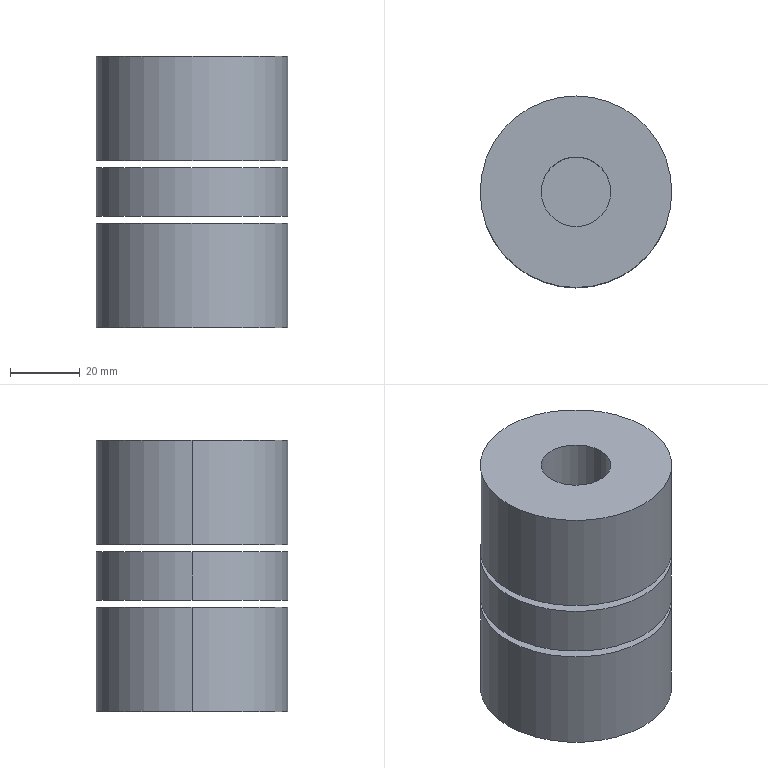Part | SolidWorks | features ICE 3, Extrusion 1 | 3 solids | 16 faces | box 55 x 55 x 78 mm | volume 157881 mm3 | cylinder 10 | plane 6 | commonest cylinder face diameters 55 x6 19 x2 20 x2
STEP:
#1=CARTESIAN_POINT('',(10.,0.,48.));
#2=VERTEX_POINT('',#1);
#3=CARTESIAN_POINT('',(-10.,0.,48.));
#4=VERTEX_POINT('',#3);
#5=CARTESIAN_POINT('',(0.,0.,48.));
#6=DIRECTION('',(0.,0.,-1.));
#7=DIRECTION('',(1.,0.,0.));
#8=AXIS2_PLACEMENT_3D('',#5,#6,#7);
#9=CIRCLE('',#8,10.);
#10=EDGE_CURVE('',#2,#4,#9,.T.);
#11=ORIENTED_EDGE('',*,*,#10,.T.);
#12=CARTESIAN_POINT('',(-10.,0.,78.));
#13=VERTEX_POINT('',#12);
#14=CARTESIAN_POINT('',(-10.,0.,48.));
#15=DIRECTION('',(0.,0.,1.));
#16=VECTOR('',#15,1000.);
#17=LINE('',#14,#16);
#18=EDGE_CURVE('',#4,#13,#17,.T.);
#19=ORIENTED_EDGE('',*,*,#18,.T.);
#20=CARTESIAN_POINT('',(10.,0.,78.));
#21=VERTEX_POINT('',#20);
#22=CARTESIAN_POINT('',(0.,0.,78.));
#23=DIRECTION('',(0.,0.,1.));
#24=DIRECTION('',(1.,0.,0.));
#25=AXIS2_PLACEMENT_3D('',#22,#23,#24);
#26=CIRCLE('',#25,10.);
#27=EDGE_CURVE('',#13,#21,#26,.T.);
#28=ORIENTED_EDGE('',*,*,#27,.T.);
#29=CARTESIAN_POINT('',(10.,0.,48.));
#30=DIRECTION('',(0.,0.,1.));
#31=VECTOR('',#30,1000.);
#32=LINE('',#29,#31);
#33=EDGE_CURVE('',#2,#21,#32,.T.);
#34=ORIENTED_EDGE('',*,*,#33,.F.);
#35=EDGE_LOOP('',(#11,#19,#28,#34));
#36=FACE_OUTER_BOUND('',#35,.T.);
#37=CARTESIAN_POINT('',(0.,0.,48.));
#38=DIRECTION('',(0.,0.,1.));
#39=DIRECTION('',(1.,0.,0.));
#40=AXIS2_PLACEMENT_3D('',#37,#38,#39);
#41=CYLINDRICAL_SURFACE('',#40,10.);
#42=ADVANCED_FACE('',(#36),#41,.F.);
#43=CARTESIAN_POINT('',(27.5,0.,78.));
#44=VERTEX_POINT('',#43);
#45=CARTESIAN_POINT('',(-27.5,0.,78.));
#46=VERTEX_POINT('',#45);
#47=CARTESIAN_POINT('',(0.,0.,78.));
#48=DIRECTION('',(0.,0.,1.));
#49=DIRECTION('',(1.,0.,0.));
#50=AXIS2_PLACEMENT_3D('',#47,#48,#49);
#51=CIRCLE('',#50,27.5);
#52=EDGE_CURVE('',#44,#46,#51,.T.);
#53=ORIENTED_EDGE('',*,*,#52,.F.);
#54=CARTESIAN_POINT('',(27.5,0.,48.));
#55=VERTEX_POINT('',#54);
#56=CARTESIAN_POINT('',(27.5,0.,78.));
#57=DIRECTION('',(0.,0.,-1.));
#58=VECTOR('',#57,1000.);
#59=LINE('',#56,#58);
#60=EDGE_CURVE('',#44,#55,#59,.T.);
#61=ORIENTED_EDGE('',*,*,#60,.T.);
#62=CARTESIAN_POINT('',(-27.5,0.,48.));
#63=VERTEX_POINT('',#62);
#64=CARTESIAN_POINT('',(0.,0.,48.));
#65=DIRECTION('',(0.,0.,1.));
#66=DIRECTION('',(1.,0.,0.));
#67=AXIS2_PLACEMENT_3D('',#64,#65,#66);
#68=CIRCLE('',#67,27.5);
#69=EDGE_CURVE('',#55,#63,#68,.T.);
#70=ORIENTED_EDGE('',*,*,#69,.T.);
#71=CARTESIAN_POINT('',(-27.5,0.,78.));
#72=DIRECTION('',(0.,0.,-1.));
#73=VECTOR('',#72,1000.);
#74=LINE('',#71,#73);
#75=EDGE_CURVE('',#46,#63,#74,.T.);
#76=ORIENTED_EDGE('',*,*,#75,.F.);
#77=EDGE_LOOP('',(#53,#61,#70,#76));
#78=FACE_OUTER_BOUND('',#77,.T.);
#79=CARTESIAN_POINT('',(0.,0.,78.));
#80=DIRECTION('',(0.,0.,-1.));
#81=DIRECTION('',(-1.,0.,0.));
#82=AXIS2_PLACEMENT_3D('',#79,#80,#81);
#83=CYLINDRICAL_SURFACE('',#82,27.5);
#84=ADVANCED_FACE('',(#78),#83,.T.);
#85=ORIENTED_EDGE('',*,*,#60,.F.);
#86=CARTESIAN_POINT('',(0.,0.,78.));
#87=DIRECTION('',(0.,0.,1.));
#88=DIRECTION('',(1.,0.,0.));
#89=AXIS2_PLACEMENT_3D('',#86,#87,#88);
#90=CIRCLE('',#89,27.5);
#91=EDGE_CURVE('',#46,#44,#90,.T.);
#92=ORIENTED_EDGE('',*,*,#91,.F.);
#93=ORIENTED_EDGE('',*,*,#75,.T.);
#94=CARTESIAN_POINT('',(0.,0.,48.));
#95=DIRECTION('',(0.,0.,1.));
#96=DIRECTION('',(1.,0.,0.));
#97=AXIS2_PLACEMENT_3D('',#94,#95,#96);
#98=CIRCLE('',#97,27.5);
#99=EDGE_CURVE('',#63,#55,#98,.T.);
#100=ORIENTED_EDGE('',*,*,#99,.T.);
#101=EDGE_LOOP('',(#85,#92,#93,#100));
#102=FACE_OUTER_BOUND('',#101,.T.);
#103=CARTESIAN_POINT('',(0.,0.,78.));
#104=DIRECTION('',(0.,0.,-1.));
#105=DIRECTION('',(-1.,0.,0.));
#106=AXIS2_PLACEMENT_3D('',#103,#104,#105);
#107=CYLINDRICAL_SURFACE('',#106,27.5);
#108=ADVANCED_FACE('',(#102),#107,.T.);
#109=CARTESIAN_POINT('',(0.,0.,78.));
#110=DIRECTION('',(0.,0.,1.));
#111=DIRECTION('',(1.,0.,0.));
#112=AXIS2_PLACEMENT_3D('',#109,#110,#111);
#113=CIRCLE('',#112,10.);
#114=EDGE_CURVE('',#21,#13,#113,.T.);
#115=ORIENTED_EDGE('',*,*,#114,.F.);
#116=ORIENTED_EDGE('',*,*,#27,.F.);
#117=EDGE_LOOP('',(#115,#116));
#118=FACE_BOUND('',#117,.T.);
#119=ORIENTED_EDGE('',*,*,#91,.T.);
#120=ORIENTED_EDGE('',*,*,#52,.T.);
#121=EDGE_LOOP('',(#119,#120));
#122=FACE_OUTER_BOUND('',#121,.T.);
#123=CARTESIAN_POINT('',(0.,0.,78.));
#124=DIRECTION('',(0.,0.,1.));
#125=DIRECTION('',(1.,0.,0.));
#126=AXIS2_PLACEMENT_3D('',#123,#124,#125);
#127=PLANE('',#126);
#128=ADVANCED_FACE('',(#118,#122),#127,.T.);
#129=ORIENTED_EDGE('',*,*,#18,.F.);
#130=CARTESIAN_POINT('',(0.,0.,48.));
#131=DIRECTION('',(0.,0.,-1.));
#132=DIRECTION('',(1.,0.,0.));
#133=AXIS2_PLACEMENT_3D('',#130,#131,#132);
#134=CIRCLE('',#133,10.);
#135=EDGE_CURVE('',#4,#2,#134,.T.);
#136=ORIENTED_EDGE('',*,*,#135,.T.);
#137=ORIENTED_EDGE('',*,*,#33,.T.);
#138=ORIENTED_EDGE('',*,*,#114,.T.);
#139=EDGE_LOOP('',(#129,#136,#137,#138));
#140=FACE_OUTER_BOUND('',#139,.T.);
#141=CARTESIAN_POINT('',(0.,0.,48.));
#142=DIRECTION('',(0.,0.,1.));
#143=DIRECTION('',(1.,0.,0.));
#144=AXIS2_PLACEMENT_3D('',#141,#142,#143);
#145=CYLINDRICAL_SURFACE('',#144,10.);
#146=ADVANCED_FACE('',(#140),#145,.F.);
#147=ORIENTED_EDGE('',*,*,#10,.F.);
#148=ORIENTED_EDGE('',*,*,#135,.F.);
#149=EDGE_LOOP('',(#147,#148));
#150=FACE_BOUND('',#149,.T.);
#151=ORIENTED_EDGE('',*,*,#99,.F.);
#152=ORIENTED_EDGE('',*,*,#69,.F.);
#153=EDGE_LOOP('',(#151,#152));
#154=FACE_OUTER_BOUND('',#153,.T.);
#155=CARTESIAN_POINT('',(-29.759,-30.,48.));
#156=DIRECTION('',(0.,0.,1.));
#157=DIRECTION('',(1.,0.,0.));
#158=AXIS2_PLACEMENT_3D('',#155,#156,#157);
#159=PLANE('',#158);
#160=ADVANCED_FACE('',(#150,#154),#159,.F.);
#161=CLOSED_SHELL('',(#42,#84,#108,#128,#146,#160));
#162=MANIFOLD_SOLID_BREP('',#161);
#163=CARTESIAN_POINT('',(-9.5,0.,30.));
#164=VERTEX_POINT('',#163);
#165=CARTESIAN_POINT('',(9.5,0.,30.));
#166=VERTEX_POINT('',#165);
#167=CARTESIAN_POINT('',(0.,0.,30.));
#168=DIRECTION('',(0.,0.,1.));
#169=DIRECTION('',(-1.,0.,0.));
#170=AXIS2_PLACEMENT_3D('',#167,#168,#169);
#171=CIRCLE('',#170,9.5);
#172=EDGE_CURVE('',#164,#166,#171,.T.);
#173=ORIENTED_EDGE('',*,*,#172,.T.);
#174=CARTESIAN_POINT('',(9.5,0.,0.));
#175=VERTEX_POINT('',#174);
#176=CARTESIAN_POINT('',(9.5,0.,30.));
#177=DIRECTION('',(0.,0.,-1.));
#178=VECTOR('',#177,1000.);
#179=LINE('',#176,#178);
#180=EDGE_CURVE('',#166,#175,#179,.T.);
#181=ORIENTED_EDGE('',*,*,#180,.T.);
#182=CARTESIAN_POINT('',(-9.5,0.,0.));
#183=VERTEX_POINT('',#182);
#184=CARTESIAN_POINT('',(0.,0.,0.));
#185=DIRECTION('',(0.,0.,-1.));
#186=DIRECTION('',(-1.,0.,0.));
#187=AXIS2_PLACEMENT_3D('',#184,#185,#186);
#188=CIRCLE('',#187,9.5);
#189=EDGE_CURVE('',#175,#183,#188,.T.);
#190=ORIENTED_EDGE('',*,*,#189,.T.);
#191=CARTESIAN_POINT('',(-9.5,0.,30.));
#192=DIRECTION('',(0.,0.,-1.));
#193=VECTOR('',#192,1000.);
#194=LINE('',#191,#193);
#195=EDGE_CURVE('',#164,#183,#194,.T.);
#196=ORIENTED_EDGE('',*,*,#195,.F.);
#197=EDGE_LOOP('',(#173,#181,#190,#196));
#198=FACE_OUTER_BOUND('',#197,.T.);
#199=CARTESIAN_POINT('',(0.,0.,30.));
#200=DIRECTION('',(0.,0.,-1.));
#201=DIRECTION('',(-1.,0.,0.));
#202=AXIS2_PLACEMENT_3D('',#199,#200,#201);
#203=CYLINDRICAL_SURFACE('',#202,9.5);
#204=ADVANCED_FACE('',(#198),#203,.F.);
#205=CARTESIAN_POINT('',(-27.5,0.,30.));
#206=VERTEX_POINT('',#205);
#207=CARTESIAN_POINT('',(27.5,0.,30.));
#208=VERTEX_POINT('',#207);
#209=CARTESIAN_POINT('',(0.,0.,30.));
#210=DIRECTION('',(0.,0.,-1.));
#211=DIRECTION('',(-1.,0.,0.));
#212=AXIS2_PLACEMENT_3D('',#209,#210,#211);
#213=CIRCLE('',#212,27.5);
#214=EDGE_CURVE('',#206,#208,#213,.T.);
#215=ORIENTED_EDGE('',*,*,#214,.T.);
#216=CARTESIAN_POINT('',(27.5,0.,0.));
#217=VERTEX_POINT('',#216);
#218=CARTESIAN_POINT('',(27.5,0.,78.));
#219=DIRECTION('',(0.,0.,-1.));
#220=VECTOR('',#219,1000.);
#221=LINE('',#218,#220);
#222=EDGE_CURVE('',#208,#217,#221,.T.);
#223=ORIENTED_EDGE('',*,*,#222,.T.);
#224=CARTESIAN_POINT('',(-27.5,0.,0.));
#225=VERTEX_POINT('',#224);
#226=CARTESIAN_POINT('',(0.,0.,0.));
#227=DIRECTION('',(0.,0.,1.));
#228=DIRECTION('',(1.,0.,0.));
#229=AXIS2_PLACEMENT_3D('',#226,#227,#228);
#230=CIRCLE('',#229,27.5);
#231=EDGE_CURVE('',#217,#225,#230,.T.);
#232=ORIENTED_EDGE('',*,*,#231,.T.);
#233=CARTESIAN_POINT('',(-27.5,0.,78.));
#234=DIRECTION('',(0.,0.,-1.));
#235=VECTOR('',#234,1000.);
#236=LINE('',#233,#235);
#237=EDGE_CURVE('',#206,#225,#236,.T.);
#238=ORIENTED_EDGE('',*,*,#237,.F.);
#239=EDGE_LOOP('',(#215,#223,#232,#238));
#240=FACE_OUTER_BOUND('',#239,.T.);
#241=CARTESIAN_POINT('',(0.,0.,78.));
#242=DIRECTION('',(0.,0.,-1.));
#243=DIRECTION('',(-1.,0.,0.));
#244=AXIS2_PLACEMENT_3D('',#241,#242,#243);
#245=CYLINDRICAL_SURFACE('',#244,27.5);
#246=ADVANCED_FACE('',(#240),#245,.T.);
#247=ORIENTED_EDGE('',*,*,#222,.F.);
#248=CARTESIAN_POINT('',(0.,0.,30.));
#249=DIRECTION('',(0.,0.,-1.));
#250=DIRECTION('',(-1.,0.,0.));
#251=AXIS2_PLACEMENT_3D('',#248,#249,#250);
#252=CIRCLE('',#251,27.5);
#253=EDGE_CURVE('',#208,#206,#252,.T.);
#254=ORIENTED_EDGE('',*,*,#253,.T.);
#255=ORIENTED_EDGE('',*,*,#237,.T.);
#256=CARTESIAN_POINT('',(0.,0.,0.));
#257=DIRECTION('',(0.,0.,1.));
#258=DIRECTION('',(1.,0.,0.));
#259=AXIS2_PLACEMENT_3D('',#256,#257,#258);
#260=CIRCLE('',#259,27.5);
#261=EDGE_CURVE('',#225,#217,#260,.T.);
#262=ORIENTED_EDGE('',*,*,#261,.T.);
#263=EDGE_LOOP('',(#247,#254,#255,#262));
#264=FACE_OUTER_BOUND('',#263,.T.);
#265=CARTESIAN_POINT('',(0.,0.,78.));
#266=DIRECTION('',(0.,0.,-1.));
#267=DIRECTION('',(-1.,0.,0.));
#268=AXIS2_PLACEMENT_3D('',#265,#266,#267);
#269=CYLINDRICAL_SURFACE('',#268,27.5);
#270=ADVANCED_FACE('',(#264),#269,.T.);
#271=CARTESIAN_POINT('',(0.,0.,0.));
#272=DIRECTION('',(0.,0.,-1.));
#273=DIRECTION('',(-1.,0.,0.));
#274=AXIS2_PLACEMENT_3D('',#271,#272,#273);
#275=CIRCLE('',#274,9.5);
#276=EDGE_CURVE('',#183,#175,#275,.T.);
#277=ORIENTED_EDGE('',*,*,#276,.F.);
#278=ORIENTED_EDGE('',*,*,#189,.F.);
#279=EDGE_LOOP('',(#277,#278));
#280=FACE_BOUND('',#279,.T.);
#281=ORIENTED_EDGE('',*,*,#261,.F.);
#282=ORIENTED_EDGE('',*,*,#231,.F.);
#283=EDGE_LOOP('',(#281,#282));
#284=FACE_OUTER_BOUND('',#283,.T.);
#285=CARTESIAN_POINT('',(0.,0.,0.));
#286=DIRECTION('',(0.,0.,1.));
#287=DIRECTION('',(1.,0.,0.));
#288=AXIS2_PLACEMENT_3D('',#285,#286,#287);
#289=PLANE('',#288);
#290=ADVANCED_FACE('',(#280,#284),#289,.F.);
#291=ORIENTED_EDGE('',*,*,#180,.F.);
#292=CARTESIAN_POINT('',(0.,0.,30.));
#293=DIRECTION('',(0.,0.,1.));
#294=DIRECTION('',(-1.,0.,0.));
#295=AXIS2_PLACEMENT_3D('',#292,#293,#294);
#296=CIRCLE('',#295,9.5);
#297=EDGE_CURVE('',#166,#164,#296,.T.);
#298=ORIENTED_EDGE('',*,*,#297,.T.);
#299=ORIENTED_EDGE('',*,*,#195,.T.);
#300=ORIENTED_EDGE('',*,*,#276,.T.);
#301=EDGE_LOOP('',(#291,#298,#299,#300));
#302=FACE_OUTER_BOUND('',#301,.T.);
#303=CARTESIAN_POINT('',(0.,0.,30.));
#304=DIRECTION('',(0.,0.,-1.));
#305=DIRECTION('',(-1.,0.,0.));
#306=AXIS2_PLACEMENT_3D('',#303,#304,#305);
#307=CYLINDRICAL_SURFACE('',#306,9.5);
#308=ADVANCED_FACE('',(#302),#307,.F.);
#309=ORIENTED_EDGE('',*,*,#172,.F.);
#310=ORIENTED_EDGE('',*,*,#297,.F.);
#311=EDGE_LOOP('',(#309,#310));
#312=FACE_BOUND('',#311,.T.);
#313=ORIENTED_EDGE('',*,*,#214,.F.);
#314=ORIENTED_EDGE('',*,*,#253,.F.);
#315=EDGE_LOOP('',(#313,#314));
#316=FACE_OUTER_BOUND('',#315,.T.);
#317=CARTESIAN_POINT('',(-29.759,-30.,30.));
#318=DIRECTION('',(0.,0.,-1.));
#319=DIRECTION('',(-1.,0.,0.));
#320=AXIS2_PLACEMENT_3D('',#317,#318,#319);
#321=PLANE('',#320);
#322=ADVANCED_FACE('',(#312,#316),#321,.F.);
#323=CLOSED_SHELL('',(#204,#246,#270,#290,#308,#322));
#324=MANIFOLD_SOLID_BREP('',#323);
#325=CARTESIAN_POINT('',(-27.5,0.,46.));
#326=VERTEX_POINT('',#325);
#327=CARTESIAN_POINT('',(27.5,0.,46.));
#328=VERTEX_POINT('',#327);
#329=CARTESIAN_POINT('',(0.,0.,46.));
#330=DIRECTION('',(0.,0.,-1.));
#331=DIRECTION('',(-1.,0.,0.));
#332=AXIS2_PLACEMENT_3D('',#329,#330,#331);
#333=CIRCLE('',#332,27.5);
#334=EDGE_CURVE('',#326,#328,#333,.T.);
#335=ORIENTED_EDGE('',*,*,#334,.T.);
#336=CARTESIAN_POINT('',(27.5,0.,32.));
#337=VERTEX_POINT('',#336);
#338=CARTESIAN_POINT('',(27.5,0.,78.));
#339=DIRECTION('',(0.,0.,-1.));
#340=VECTOR('',#339,1000.);
#341=LINE('',#338,#340);
#342=EDGE_CURVE('',#328,#337,#341,.T.);
#343=ORIENTED_EDGE('',*,*,#342,.T.);
#344=CARTESIAN_POINT('',(-27.5,0.,32.));
#345=VERTEX_POINT('',#344);
#346=CARTESIAN_POINT('',(0.,0.,32.));
#347=DIRECTION('',(0.,0.,1.));
#348=DIRECTION('',(1.,0.,0.));
#349=AXIS2_PLACEMENT_3D('',#346,#347,#348);
#350=CIRCLE('',#349,27.5);
#351=EDGE_CURVE('',#337,#345,#350,.T.);
#352=ORIENTED_EDGE('',*,*,#351,.T.);
#353=CARTESIAN_POINT('',(-27.5,0.,78.));
#354=DIRECTION('',(0.,0.,-1.));
#355=VECTOR('',#354,1000.);
#356=LINE('',#353,#355);
#357=EDGE_CURVE('',#326,#345,#356,.T.);
#358=ORIENTED_EDGE('',*,*,#357,.F.);
#359=EDGE_LOOP('',(#335,#343,#352,#358));
#360=FACE_OUTER_BOUND('',#359,.T.);
#361=CARTESIAN_POINT('',(0.,0.,78.));
#362=DIRECTION('',(0.,0.,-1.));
#363=DIRECTION('',(-1.,0.,0.));
#364=AXIS2_PLACEMENT_3D('',#361,#362,#363);
#365=CYLINDRICAL_SURFACE('',#364,27.5);
#366=ADVANCED_FACE('',(#360),#365,.T.);
#367=ORIENTED_EDGE('',*,*,#342,.F.);
#368=CARTESIAN_POINT('',(0.,0.,46.));
#369=DIRECTION('',(0.,0.,-1.));
#370=DIRECTION('',(-1.,0.,0.));
#371=AXIS2_PLACEMENT_3D('',#368,#369,#370);
#372=CIRCLE('',#371,27.5);
#373=EDGE_CURVE('',#328,#326,#372,.T.);
#374=ORIENTED_EDGE('',*,*,#373,.T.);
#375=ORIENTED_EDGE('',*,*,#357,.T.);
#376=CARTESIAN_POINT('',(0.,0.,32.));
#377=DIRECTION('',(0.,0.,1.));
#378=DIRECTION('',(1.,0.,0.));
#379=AXIS2_PLACEMENT_3D('',#376,#377,#378);
#380=CIRCLE('',#379,27.5);
#381=EDGE_CURVE('',#345,#337,#380,.T.);
#382=ORIENTED_EDGE('',*,*,#381,.T.);
#383=EDGE_LOOP('',(#367,#374,#375,#382));
#384=FACE_OUTER_BOUND('',#383,.T.);
#385=CARTESIAN_POINT('',(0.,0.,78.));
#386=DIRECTION('',(0.,0.,-1.));
#387=DIRECTION('',(-1.,0.,0.));
#388=AXIS2_PLACEMENT_3D('',#385,#386,#387);
#389=CYLINDRICAL_SURFACE('',#388,27.5);
#390=ADVANCED_FACE('',(#384),#389,.T.);
#391=ORIENTED_EDGE('',*,*,#381,.F.);
#392=ORIENTED_EDGE('',*,*,#351,.F.);
#393=EDGE_LOOP('',(#391,#392));
#394=FACE_OUTER_BOUND('',#393,.T.);
#395=CARTESIAN_POINT('',(-29.759,-30.,32.));
#396=DIRECTION('',(0.,0.,1.));
#397=DIRECTION('',(1.,0.,0.));
#398=AXIS2_PLACEMENT_3D('',#395,#396,#397);
#399=PLANE('',#398);
#400=ADVANCED_FACE('',(#394),#399,.F.);
#401=ORIENTED_EDGE('',*,*,#334,.F.);
#402=ORIENTED_EDGE('',*,*,#373,.F.);
#403=EDGE_LOOP('',(#401,#402));
#404=FACE_OUTER_BOUND('',#403,.T.);
#405=CARTESIAN_POINT('',(-29.759,-30.,46.));
#406=DIRECTION('',(0.,0.,-1.));
#407=DIRECTION('',(-1.,0.,0.));
#408=AXIS2_PLACEMENT_3D('',#405,#406,#407);
#409=PLANE('',#408);
#410=ADVANCED_FACE('',(#404),#409,.F.);
#411=CLOSED_SHELL('',(#366,#390,#400,#410));
#412=MANIFOLD_SOLID_BREP('',#411);
#413=CARTESIAN_POINT('',(0.,0.,0.));
#414=DIRECTION('',(0.,0.,1.));
#415=DIRECTION('',(1.,0.,0.));
#416=AXIS2_PLACEMENT_3D('',#413,#414,#415);
#417=(LENGTH_UNIT()NAMED_UNIT(*)SI_UNIT(.MILLI.,.METRE.));
#418=UNCERTAINTY_MEASURE_WITH_UNIT(LENGTH_MEASURE(0.00001),#417,'','');
#419=(NAMED_UNIT(*)PLANE_ANGLE_UNIT()SI_UNIT($,.RADIAN.));
#420=(NAMED_UNIT(*)SI_UNIT($,.STERADIAN.)SOLID_ANGLE_UNIT());
#421=(GEOMETRIC_REPRESENTATION_CONTEXT(3)GLOBAL_UNCERTAINTY_ASSIGNED_CONTEXT((#418))GLOBAL_UNIT_ASSIGNED_CONTEXT((#417,#419,#420))REPRESENTATION_CONTEXT('',''));
#422=ADVANCED_BREP_SHAPE_REPRESENTATION('',(#162,#324,#412,#416),#421);